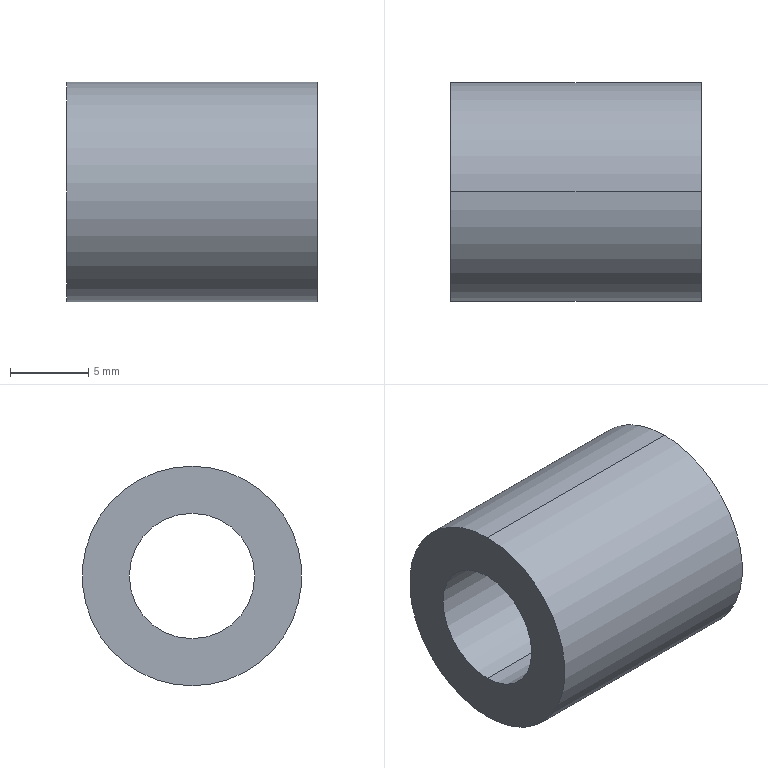Part | SolidWorks | features Revolution 1 | 1 solid | 8 faces | box 16 x 14 x 14 mm | volume 1434 mm3 | cylinder 4 | cone 2 | plane 2 | commonest cylinder face diameters 8 x2 14 x2
STEP:
#1=CARTESIAN_POINT('',(16.,0.,7.));
#2=VERTEX_POINT('',#1);
#3=CARTESIAN_POINT('',(16.,0.,-7.));
#4=VERTEX_POINT('',#3);
#5=CARTESIAN_POINT('',(16.,0.,0.));
#6=DIRECTION('',(-1.,0.,0.));
#7=DIRECTION('',(0.,0.,1.));
#8=AXIS2_PLACEMENT_3D('',#5,#6,#7);
#9=CIRCLE('',#8,7.);
#10=EDGE_CURVE('',#2,#4,#9,.T.);
#11=ORIENTED_EDGE('',*,*,#10,.T.);
#12=CARTESIAN_POINT('',(0.,0.,-7.));
#13=VERTEX_POINT('',#12);
#14=CARTESIAN_POINT('',(0.,0.,-7.));
#15=DIRECTION('',(-1.,0.,0.));
#16=VECTOR('',#15,1000.);
#17=LINE('',#14,#16);
#18=EDGE_CURVE('',#4,#13,#17,.T.);
#19=ORIENTED_EDGE('',*,*,#18,.T.);
#20=CARTESIAN_POINT('',(0.,0.,7.));
#21=VERTEX_POINT('',#20);
#22=CARTESIAN_POINT('',(0.,0.,0.));
#23=DIRECTION('',(-1.,0.,0.));
#24=DIRECTION('',(0.,0.,1.));
#25=AXIS2_PLACEMENT_3D('',#22,#23,#24);
#26=CIRCLE('',#25,7.);
#27=EDGE_CURVE('',#21,#13,#26,.T.);
#28=ORIENTED_EDGE('',*,*,#27,.F.);
#29=CARTESIAN_POINT('',(0.,0.,7.));
#30=DIRECTION('',(-1.,0.,0.));
#31=VECTOR('',#30,1000.);
#32=LINE('',#29,#31);
#33=EDGE_CURVE('',#2,#21,#32,.T.);
#34=ORIENTED_EDGE('',*,*,#33,.F.);
#35=EDGE_LOOP('',(#11,#19,#28,#34));
#36=FACE_OUTER_BOUND('',#35,.T.);
#37=CARTESIAN_POINT('',(0.,0.,0.));
#38=DIRECTION('',(-1.,0.,0.));
#39=DIRECTION('',(0.,0.,1.));
#40=AXIS2_PLACEMENT_3D('',#37,#38,#39);
#41=CYLINDRICAL_SURFACE('',#40,7.);
#42=ADVANCED_FACE('',(#36),#41,.T.);
#43=CARTESIAN_POINT('',(11.,0.,-4.));
#44=VERTEX_POINT('',#43);
#45=CARTESIAN_POINT('',(11.,0.,4.));
#46=VERTEX_POINT('',#45);
#47=CARTESIAN_POINT('',(11.,0.,0.));
#48=DIRECTION('',(-1.,0.,0.));
#49=DIRECTION('',(0.,0.,1.));
#50=AXIS2_PLACEMENT_3D('',#47,#48,#49);
#51=CIRCLE('',#50,4.);
#52=EDGE_CURVE('',#44,#46,#51,.T.);
#53=ORIENTED_EDGE('',*,*,#52,.T.);
#54=CARTESIAN_POINT('',(16.,0.,6.887));
#55=VERTEX_POINT('',#54);
#56=CARTESIAN_POINT('',(11.,0.,4.));
#57=DIRECTION('',(0.866,0.,0.5));
#58=VECTOR('',#57,1000.);
#59=LINE('',#56,#58);
#60=EDGE_CURVE('',#46,#55,#59,.T.);
#61=ORIENTED_EDGE('',*,*,#60,.T.);
#62=CARTESIAN_POINT('',(16.,0.,-6.887));
#63=VERTEX_POINT('',#62);
#64=CARTESIAN_POINT('',(16.,0.,0.));
#65=DIRECTION('',(-1.,0.,0.));
#66=DIRECTION('',(0.,0.,1.));
#67=AXIS2_PLACEMENT_3D('',#64,#65,#66);
#68=CIRCLE('',#67,6.887);
#69=EDGE_CURVE('',#63,#55,#68,.T.);
#70=ORIENTED_EDGE('',*,*,#69,.F.);
#71=CARTESIAN_POINT('',(11.,0.,-4.));
#72=DIRECTION('',(0.866,0.,-0.5));
#73=VECTOR('',#72,1000.);
#74=LINE('',#71,#73);
#75=EDGE_CURVE('',#44,#63,#74,.T.);
#76=ORIENTED_EDGE('',*,*,#75,.F.);
#77=EDGE_LOOP('',(#53,#61,#70,#76));
#78=FACE_OUTER_BOUND('',#77,.T.);
#79=CARTESIAN_POINT('',(11.,0.,0.));
#80=DIRECTION('',(1.,0.,0.));
#81=DIRECTION('',(0.,0.,-1.));
#82=AXIS2_PLACEMENT_3D('',#79,#80,#81);
#83=CONICAL_SURFACE('',#82,4.,0.5236);
#84=ADVANCED_FACE('',(#78),#83,.F.);
#85=ORIENTED_EDGE('',*,*,#52,.F.);
#86=CARTESIAN_POINT('',(0.,0.,-4.));
#87=VERTEX_POINT('',#86);
#88=CARTESIAN_POINT('',(0.,0.,-4.));
#89=DIRECTION('',(-1.,0.,0.));
#90=VECTOR('',#89,1000.);
#91=LINE('',#88,#90);
#92=EDGE_CURVE('',#44,#87,#91,.T.);
#93=ORIENTED_EDGE('',*,*,#92,.T.);
#94=CARTESIAN_POINT('',(0.,0.,4.));
#95=VERTEX_POINT('',#94);
#96=CARTESIAN_POINT('',(0.,0.,0.));
#97=DIRECTION('',(-1.,0.,0.));
#98=DIRECTION('',(0.,0.,1.));
#99=AXIS2_PLACEMENT_3D('',#96,#97,#98);
#100=CIRCLE('',#99,4.);
#101=EDGE_CURVE('',#87,#95,#100,.T.);
#102=ORIENTED_EDGE('',*,*,#101,.T.);
#103=CARTESIAN_POINT('',(0.,0.,4.));
#104=DIRECTION('',(-1.,0.,0.));
#105=VECTOR('',#104,1000.);
#106=LINE('',#103,#105);
#107=EDGE_CURVE('',#46,#95,#106,.T.);
#108=ORIENTED_EDGE('',*,*,#107,.F.);
#109=EDGE_LOOP('',(#85,#93,#102,#108));
#110=FACE_OUTER_BOUND('',#109,.T.);
#111=CARTESIAN_POINT('',(0.,0.,0.));
#112=DIRECTION('',(-1.,0.,0.));
#113=DIRECTION('',(0.,0.,1.));
#114=AXIS2_PLACEMENT_3D('',#111,#112,#113);
#115=CYLINDRICAL_SURFACE('',#114,4.);
#116=ADVANCED_FACE('',(#110),#115,.F.);
#117=CARTESIAN_POINT('',(0.,0.,0.));
#118=DIRECTION('',(-1.,0.,0.));
#119=DIRECTION('',(0.,0.,1.));
#120=AXIS2_PLACEMENT_3D('',#117,#118,#119);
#121=CIRCLE('',#120,4.);
#122=EDGE_CURVE('',#95,#87,#121,.T.);
#123=ORIENTED_EDGE('',*,*,#122,.F.);
#124=ORIENTED_EDGE('',*,*,#101,.F.);
#125=EDGE_LOOP('',(#123,#124));
#126=FACE_BOUND('',#125,.T.);
#127=ORIENTED_EDGE('',*,*,#27,.T.);
#128=CARTESIAN_POINT('',(0.,0.,0.));
#129=DIRECTION('',(-1.,0.,0.));
#130=DIRECTION('',(0.,0.,1.));
#131=AXIS2_PLACEMENT_3D('',#128,#129,#130);
#132=CIRCLE('',#131,7.);
#133=EDGE_CURVE('',#13,#21,#132,.T.);
#134=ORIENTED_EDGE('',*,*,#133,.T.);
#135=EDGE_LOOP('',(#127,#134));
#136=FACE_OUTER_BOUND('',#135,.T.);
#137=CARTESIAN_POINT('',(0.,7.,0.));
#138=DIRECTION('',(1.,0.,0.));
#139=DIRECTION('',(0.,0.,-1.));
#140=AXIS2_PLACEMENT_3D('',#137,#138,#139);
#141=PLANE('',#140);
#142=ADVANCED_FACE('',(#126,#136),#141,.F.);
#143=ORIENTED_EDGE('',*,*,#92,.F.);
#144=CARTESIAN_POINT('',(11.,0.,0.));
#145=DIRECTION('',(-1.,0.,0.));
#146=DIRECTION('',(0.,0.,1.));
#147=AXIS2_PLACEMENT_3D('',#144,#145,#146);
#148=CIRCLE('',#147,4.);
#149=EDGE_CURVE('',#46,#44,#148,.T.);
#150=ORIENTED_EDGE('',*,*,#149,.F.);
#151=ORIENTED_EDGE('',*,*,#107,.T.);
#152=ORIENTED_EDGE('',*,*,#122,.T.);
#153=EDGE_LOOP('',(#143,#150,#151,#152));
#154=FACE_OUTER_BOUND('',#153,.T.);
#155=CARTESIAN_POINT('',(0.,0.,0.));
#156=DIRECTION('',(-1.,0.,0.));
#157=DIRECTION('',(0.,0.,1.));
#158=AXIS2_PLACEMENT_3D('',#155,#156,#157);
#159=CYLINDRICAL_SURFACE('',#158,4.);
#160=ADVANCED_FACE('',(#154),#159,.F.);
#161=ORIENTED_EDGE('',*,*,#60,.F.);
#162=ORIENTED_EDGE('',*,*,#149,.T.);
#163=ORIENTED_EDGE('',*,*,#75,.T.);
#164=CARTESIAN_POINT('',(16.,0.,0.));
#165=DIRECTION('',(-1.,0.,0.));
#166=DIRECTION('',(0.,0.,1.));
#167=AXIS2_PLACEMENT_3D('',#164,#165,#166);
#168=CIRCLE('',#167,6.887);
#169=EDGE_CURVE('',#55,#63,#168,.T.);
#170=ORIENTED_EDGE('',*,*,#169,.F.);
#171=EDGE_LOOP('',(#161,#162,#163,#170));
#172=FACE_OUTER_BOUND('',#171,.T.);
#173=CARTESIAN_POINT('',(11.,0.,0.));
#174=DIRECTION('',(1.,0.,0.));
#175=DIRECTION('',(0.,0.,-1.));
#176=AXIS2_PLACEMENT_3D('',#173,#174,#175);
#177=CONICAL_SURFACE('',#176,4.,0.5236);
#178=ADVANCED_FACE('',(#172),#177,.F.);
#179=ORIENTED_EDGE('',*,*,#10,.F.);
#180=CARTESIAN_POINT('',(16.,0.,0.));
#181=DIRECTION('',(-1.,0.,0.));
#182=DIRECTION('',(0.,0.,1.));
#183=AXIS2_PLACEMENT_3D('',#180,#181,#182);
#184=CIRCLE('',#183,7.);
#185=EDGE_CURVE('',#4,#2,#184,.T.);
#186=ORIENTED_EDGE('',*,*,#185,.F.);
#187=EDGE_LOOP('',(#179,#186));
#188=FACE_OUTER_BOUND('',#187,.T.);
#189=ORIENTED_EDGE('',*,*,#69,.T.);
#190=ORIENTED_EDGE('',*,*,#169,.T.);
#191=EDGE_LOOP('',(#189,#190));
#192=FACE_BOUND('',#191,.T.);
#193=CARTESIAN_POINT('',(16.,6.887,0.));
#194=DIRECTION('',(-1.,0.,0.));
#195=DIRECTION('',(0.,0.,1.));
#196=AXIS2_PLACEMENT_3D('',#193,#194,#195);
#197=PLANE('',#196);
#198=ADVANCED_FACE('',(#188,#192),#197,.F.);
#199=ORIENTED_EDGE('',*,*,#18,.F.);
#200=ORIENTED_EDGE('',*,*,#185,.T.);
#201=ORIENTED_EDGE('',*,*,#33,.T.);
#202=ORIENTED_EDGE('',*,*,#133,.F.);
#203=EDGE_LOOP('',(#199,#200,#201,#202));
#204=FACE_OUTER_BOUND('',#203,.T.);
#205=CARTESIAN_POINT('',(0.,0.,0.));
#206=DIRECTION('',(-1.,0.,0.));
#207=DIRECTION('',(0.,0.,1.));
#208=AXIS2_PLACEMENT_3D('',#205,#206,#207);
#209=CYLINDRICAL_SURFACE('',#208,7.);
#210=ADVANCED_FACE('',(#204),#209,.T.);
#211=CLOSED_SHELL('',(#42,#84,#116,#142,#160,#178,#198,#210));
#212=MANIFOLD_SOLID_BREP('',#211);
#213=CARTESIAN_POINT('',(0.,0.,0.));
#214=DIRECTION('',(0.,0.,1.));
#215=DIRECTION('',(1.,0.,0.));
#216=AXIS2_PLACEMENT_3D('',#213,#214,#215);
#217=(LENGTH_UNIT()NAMED_UNIT(*)SI_UNIT(.MILLI.,.METRE.));
#218=UNCERTAINTY_MEASURE_WITH_UNIT(LENGTH_MEASURE(0.00001),#217,'','');
#219=(NAMED_UNIT(*)PLANE_ANGLE_UNIT()SI_UNIT($,.RADIAN.));
#220=(NAMED_UNIT(*)SI_UNIT($,.STERADIAN.)SOLID_ANGLE_UNIT());
#221=(GEOMETRIC_REPRESENTATION_CONTEXT(3)GLOBAL_UNCERTAINTY_ASSIGNED_CONTEXT((#218))GLOBAL_UNIT_ASSIGNED_CONTEXT((#217,#219,#220))REPRESENTATION_CONTEXT('',''));
#222=ADVANCED_BREP_SHAPE_REPRESENTATION('',(#212,#216),#221);